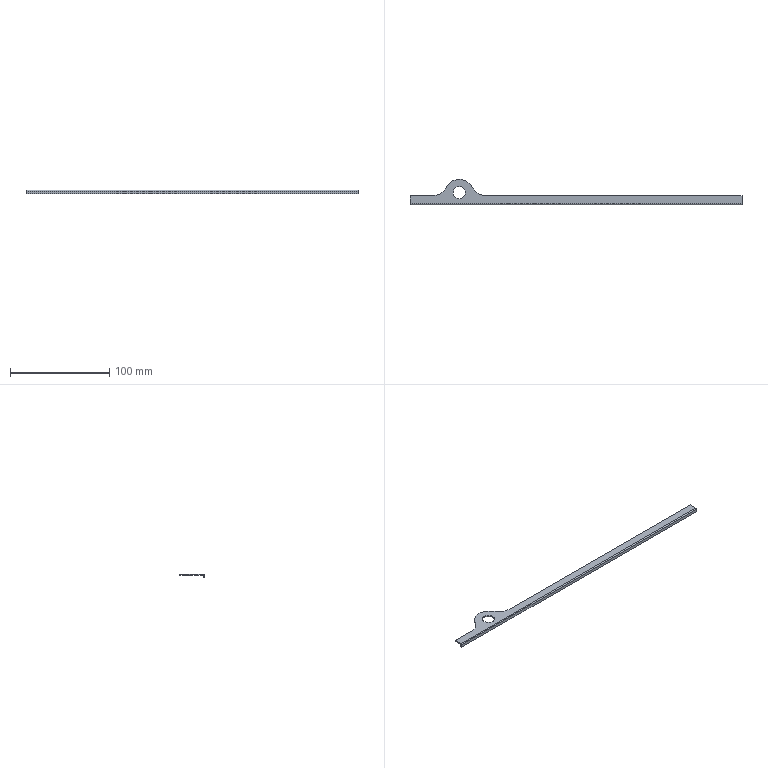Part | STEP file | gslz 2016.10.28-13_id1214_x_t | 1 solid | 14 faces | box 335 x 25.5 x 4 mm | volume 5252 mm3 | plane 9 | cylinder 5 | commonest cylinder face diameters 30 x3 2 x1 12.3 x1
STEP:
#1=CARTESIAN_POINT('',(0.,0.,0.));
#2=DIRECTION('',(0.,0.,1.));
#3=DIRECTION('',(1.,0.,0.));
#4=AXIS2_PLACEMENT_3D('',#1,#2,#3);
#5=CARTESIAN_POINT('',(-300.763,-257.,1.25));
#6=VERTEX_POINT('',#5);
#7=CARTESIAN_POINT('',(-42.345,-257.,1.25));
#8=VERTEX_POINT('',#7);
#9=CARTESIAN_POINT('',(-2539.517,-257.,1.25));
#10=DIRECTION('',(1.,0.,0.));
#11=VECTOR('',#10,1.);
#12=LINE('',#9,#11);
#13=CARTESIAN_POINT('',(-299.269,-257.,2.5));
#14=DIRECTION('',(0.,1.,0.));
#15=DIRECTION('',(-1.,0.,0.));
#16=AXIS2_PLACEMENT_3D('',#13,#14,#15);
#17=PLANE('',#16);
#18=CARTESIAN_POINT('',(2240.248,-1.25));
#19=DIRECTION('',(-1.,0.));
#20=VECTOR('',#19,1.);
#21=LINE('',#18,#20);
#22=(GEOMETRIC_REPRESENTATION_CONTEXT(2)PARAMETRIC_REPRESENTATION_CONTEXT()REPRESENTATION_CONTEXT('',''));
#23=DEFINITIONAL_REPRESENTATION('',(#21),#22);
#24=PCURVE('',#17,#23);
#25=CARTESIAN_POINT('',(-2539.517,-331.067,1.25));
#26=DIRECTION('',(0.,0.,1.));
#27=DIRECTION('',(-1.,0.,0.));
#28=AXIS2_PLACEMENT_3D('',#25,#26,#27);
#29=PLANE('',#28);
#30=CARTESIAN_POINT('',(0.,-74.067));
#31=DIRECTION('',(-1.,0.));
#32=VECTOR('',#31,1.);
#33=LINE('',#30,#32);
#34=(GEOMETRIC_REPRESENTATION_CONTEXT(2)PARAMETRIC_REPRESENTATION_CONTEXT()REPRESENTATION_CONTEXT('',''));
#35=DEFINITIONAL_REPRESENTATION('',(#33),#34);
#36=PCURVE('',#29,#35);
#37=SURFACE_CURVE('',#12,(#24,#36),.PCURVE_S1.);
#38=EDGE_CURVE('',#6,#8,#37,.T.);
#39=ORIENTED_EDGE('',*,*,#38,.T.);
#40=CARTESIAN_POINT('',(-42.345,-257.,0.));
#41=VERTEX_POINT('',#40);
#42=CARTESIAN_POINT('',(-42.345,-257.,-0.75));
#43=DIRECTION('',(0.,0.,1.));
#44=VECTOR('',#43,1.);
#45=LINE('',#42,#44);
#46=CARTESIAN_POINT('',(-256.924,-3.25));
#47=DIRECTION('',(0.,1.));
#48=VECTOR('',#47,1.);
#49=LINE('',#46,#48);
#50=(GEOMETRIC_REPRESENTATION_CONTEXT(2)PARAMETRIC_REPRESENTATION_CONTEXT()REPRESENTATION_CONTEXT('',''));
#51=DEFINITIONAL_REPRESENTATION('',(#49),#50);
#52=PCURVE('',#17,#51);
#53=CARTESIAN_POINT('',(-42.345,-261.5,-0.75));
#54=DIRECTION('',(1.,0.,0.));
#55=DIRECTION('',(0.,1.,0.));
#56=AXIS2_PLACEMENT_3D('',#53,#54,#55);
#57=PLANE('',#56);
#58=CARTESIAN_POINT('',(4.5,0.));
#59=DIRECTION('',(0.,1.));
#60=VECTOR('',#59,1.);
#61=LINE('',#58,#60);
#62=(GEOMETRIC_REPRESENTATION_CONTEXT(2)PARAMETRIC_REPRESENTATION_CONTEXT()REPRESENTATION_CONTEXT('',''));
#63=DEFINITIONAL_REPRESENTATION('',(#61),#62);
#64=PCURVE('',#57,#63);
#65=SURFACE_CURVE('',#45,(#52,#64),.PCURVE_S1.);
#66=EDGE_CURVE('',#41,#8,#65,.T.);
#67=ORIENTED_EDGE('',*,*,#66,.F.);
#68=CARTESIAN_POINT('',(-300.763,-257.,0.));
#69=VERTEX_POINT('',#68);
#70=CARTESIAN_POINT('',(-299.269,-257.,0.));
#71=DIRECTION('',(-1.,0.,0.));
#72=VECTOR('',#71,1.);
#73=LINE('',#70,#72);
#74=CARTESIAN_POINT('',(0.,-2.5));
#75=DIRECTION('',(1.,0.));
#76=VECTOR('',#75,1.);
#77=LINE('',#74,#76);
#78=(GEOMETRIC_REPRESENTATION_CONTEXT(2)PARAMETRIC_REPRESENTATION_CONTEXT()REPRESENTATION_CONTEXT('',''));
#79=DEFINITIONAL_REPRESENTATION('',(#77),#78);
#80=PCURVE('',#17,#79);
#81=CARTESIAN_POINT('',(-2539.517,-331.067,0.));
#82=DIRECTION('',(0.,0.,1.));
#83=DIRECTION('',(-1.,0.,0.));
#84=AXIS2_PLACEMENT_3D('',#81,#82,#83);
#85=PLANE('',#84);
#86=CARTESIAN_POINT('',(-2240.248,-74.067));
#87=DIRECTION('',(1.,0.));
#88=VECTOR('',#87,1.);
#89=LINE('',#86,#88);
#90=(GEOMETRIC_REPRESENTATION_CONTEXT(2)PARAMETRIC_REPRESENTATION_CONTEXT()REPRESENTATION_CONTEXT('',''));
#91=DEFINITIONAL_REPRESENTATION('',(#89),#90);
#92=PCURVE('',#85,#91);
#93=SURFACE_CURVE('',#73,(#80,#92),.PCURVE_S1.);
#94=EDGE_CURVE('',#41,#69,#93,.T.);
#95=ORIENTED_EDGE('',*,*,#94,.T.);
#96=CARTESIAN_POINT('',(-300.763,-257.,2.5));
#97=DIRECTION('',(0.,0.,1.));
#98=VECTOR('',#97,1.);
#99=LINE('',#96,#98);
#100=CARTESIAN_POINT('',(1.493,0.));
#101=DIRECTION('',(0.,1.));
#102=VECTOR('',#101,1.);
#103=LINE('',#100,#102);
#104=(GEOMETRIC_REPRESENTATION_CONTEXT(2)PARAMETRIC_REPRESENTATION_CONTEXT()REPRESENTATION_CONTEXT('',''));
#105=DEFINITIONAL_REPRESENTATION('',(#103),#104);
#106=PCURVE('',#17,#105);
#107=CARTESIAN_POINT('',(-300.763,-242.,2.5));
#108=DIRECTION('',(0.,0.,-1.));
#109=DIRECTION('',(1.,0.,0.));
#110=AXIS2_PLACEMENT_3D('',#107,#108,#109);
#111=CYLINDRICAL_SURFACE('',#110,15.);
#112=CARTESIAN_POINT('',(1.571,0.));
#113=DIRECTION('',(0.,-1.));
#114=VECTOR('',#113,1.);
#115=LINE('',#112,#114);
#116=(GEOMETRIC_REPRESENTATION_CONTEXT(2)PARAMETRIC_REPRESENTATION_CONTEXT()REPRESENTATION_CONTEXT('',''));
#117=DEFINITIONAL_REPRESENTATION('',(#115),#116);
#118=PCURVE('',#111,#117);
#119=SURFACE_CURVE('',#99,(#106,#118),.PCURVE_S1.);
#120=EDGE_CURVE('',#69,#6,#119,.T.);
#121=ORIENTED_EDGE('',*,*,#120,.T.);
#122=EDGE_LOOP('',(#39,#67,#95,#121));
#123=FACE_BOUND('',#122,.T.);
#124=ADVANCED_FACE('',(#123),#17,.T.);
#125=CARTESIAN_POINT('',(-333.704,-254.,1.25));
#126=VERTEX_POINT('',#125);
#127=CARTESIAN_POINT('',(-327.554,-254.,1.25));
#128=DIRECTION('',(0.,0.,1.));
#129=DIRECTION('',(-1.,0.,0.));
#130=AXIS2_PLACEMENT_3D('',#127,#128,#129);
#131=CIRCLE('',#130,6.15);
#132=CARTESIAN_POINT('',(-2211.964,-77.067));
#133=DIRECTION('',(1.,0.));
#134=AXIS2_PLACEMENT_2D('',#132,#133);
#135=CIRCLE('',#134,6.15);
#136=(GEOMETRIC_REPRESENTATION_CONTEXT(2)PARAMETRIC_REPRESENTATION_CONTEXT()REPRESENTATION_CONTEXT('',''));
#137=DEFINITIONAL_REPRESENTATION('',(#135),#136);
#138=PCURVE('',#29,#137);
#139=CARTESIAN_POINT('',(-327.554,-254.,2.5));
#140=DIRECTION('',(0.,0.,-1.));
#141=DIRECTION('',(1.,0.,0.));
#142=AXIS2_PLACEMENT_3D('',#139,#140,#141);
#143=CYLINDRICAL_SURFACE('',#142,6.15);
#144=CARTESIAN_POINT('',(9.425,1.25));
#145=DIRECTION('',(-1.,0.));
#146=VECTOR('',#145,1.);
#147=LINE('',#144,#146);
#148=(GEOMETRIC_REPRESENTATION_CONTEXT(2)PARAMETRIC_REPRESENTATION_CONTEXT()REPRESENTATION_CONTEXT('',''));
#149=DEFINITIONAL_REPRESENTATION('',(#147),#148);
#150=PCURVE('',#143,#149);
#151=SURFACE_CURVE('',#131,(#138,#150),.PCURVE_S1.);
#152=EDGE_CURVE('',#126,#126,#151,.T.);
#153=ORIENTED_EDGE('',*,*,#152,.F.);
#154=EDGE_LOOP('',(#153));
#155=FACE_BOUND('',#154,.T.);
#156=CARTESIAN_POINT('',(-377.345,-265.,1.25));
#157=VERTEX_POINT('',#156);
#158=CARTESIAN_POINT('',(-42.345,-265.,1.25));
#159=VERTEX_POINT('',#158);
#160=CARTESIAN_POINT('',(-119.75,-265.,1.25));
#161=DIRECTION('',(1.,0.,0.));
#162=VECTOR('',#161,1.);
#163=LINE('',#160,#162);
#164=CARTESIAN_POINT('',(-2419.767,-66.067));
#165=DIRECTION('',(-1.,0.));
#166=VECTOR('',#165,1.);
#167=LINE('',#164,#166);
#168=(GEOMETRIC_REPRESENTATION_CONTEXT(2)PARAMETRIC_REPRESENTATION_CONTEXT()REPRESENTATION_CONTEXT('',''));
#169=DEFINITIONAL_REPRESENTATION('',(#167),#168);
#170=PCURVE('',#29,#169);
#171=CARTESIAN_POINT('',(-2539.517,-265.,0.25));
#172=DIRECTION('',(1.,0.,0.));
#173=DIRECTION('',(0.,1.,0.));
#174=AXIS2_PLACEMENT_3D('',#171,#172,#173);
#175=CYLINDRICAL_SURFACE('',#174,1.);
#176=CARTESIAN_POINT('',(1.571,2419.767));
#177=DIRECTION('',(0.,1.));
#178=VECTOR('',#177,1.);
#179=LINE('',#176,#178);
#180=(GEOMETRIC_REPRESENTATION_CONTEXT(2)PARAMETRIC_REPRESENTATION_CONTEXT()REPRESENTATION_CONTEXT('',''));
#181=DEFINITIONAL_REPRESENTATION('',(#179),#180);
#182=PCURVE('',#175,#181);
#183=SURFACE_CURVE('',#163,(#170,#182),.PCURVE_S1.);
#184=EDGE_CURVE('',#157,#159,#183,.T.);
#185=ORIENTED_EDGE('',*,*,#184,.T.);
#186=CARTESIAN_POINT('',(-42.345,-331.067,1.25));
#187=DIRECTION('',(0.,1.,0.));
#188=VECTOR('',#187,1.);
#189=LINE('',#186,#188);
#190=CARTESIAN_POINT('',(-2497.172,0.));
#191=DIRECTION('',(0.,-1.));
#192=VECTOR('',#191,1.);
#193=LINE('',#190,#192);
#194=(GEOMETRIC_REPRESENTATION_CONTEXT(2)PARAMETRIC_REPRESENTATION_CONTEXT()REPRESENTATION_CONTEXT('',''));
#195=DEFINITIONAL_REPRESENTATION('',(#193),#194);
#196=PCURVE('',#29,#195);
#197=CARTESIAN_POINT('',(-69.567,2.));
#198=DIRECTION('',(1.,0.));
#199=VECTOR('',#198,1.);
#200=LINE('',#197,#199);
#201=(GEOMETRIC_REPRESENTATION_CONTEXT(2)PARAMETRIC_REPRESENTATION_CONTEXT()REPRESENTATION_CONTEXT('',''));
#202=DEFINITIONAL_REPRESENTATION('',(#200),#201);
#203=PCURVE('',#57,#202);
#204=SURFACE_CURVE('',#189,(#196,#203),.PCURVE_S1.);
#205=EDGE_CURVE('',#159,#8,#204,.T.);
#206=ORIENTED_EDGE('',*,*,#205,.T.);
#207=ORIENTED_EDGE('',*,*,#38,.F.);
#208=CARTESIAN_POINT('',(-314.158,-248.75,1.25));
#209=VERTEX_POINT('',#208);
#210=CARTESIAN_POINT('',(-300.763,-242.,1.25));
#211=DIRECTION('',(0.,0.,-1.));
#212=DIRECTION('',(-1.,0.,0.));
#213=AXIS2_PLACEMENT_3D('',#210,#211,#212);
#214=CIRCLE('',#213,15.);
#215=CARTESIAN_POINT('',(-2223.754,-89.067));
#216=CARTESIAN_POINT('',(-2223.754,-115.047));
#217=CARTESIAN_POINT('',(-2246.254,-102.057));
#218=CARTESIAN_POINT('',(-2268.754,-89.067));
#219=CARTESIAN_POINT('',(-2246.254,-76.076));
#220=CARTESIAN_POINT('',(-2223.754,-63.086));
#221=CARTESIAN_POINT('',(-2223.754,-89.067));
#222=(BOUNDED_CURVE()B_SPLINE_CURVE(2,(#215,#216,#217,#218,#219,#220,#221),.UNSPECIFIED.,.T.,.F.)B_SPLINE_CURVE_WITH_KNOTS((1,2,2,2,2,1),(-2.094,0.,2.094,4.189,6.283,8.378),.UNSPECIFIED.)CURVE()GEOMETRIC_REPRESENTATION_ITEM()RATIONAL_B_SPLINE_CURVE((1.,0.5,1.,0.5,1.,0.5,1.))REPRESENTATION_ITEM(''));
#223=(GEOMETRIC_REPRESENTATION_CONTEXT(2)PARAMETRIC_REPRESENTATION_CONTEXT()REPRESENTATION_CONTEXT('',''));
#224=DEFINITIONAL_REPRESENTATION('',(#222),#223);
#225=PCURVE('',#29,#224);
#226=CARTESIAN_POINT('',(-3.142,1.25));
#227=DIRECTION('',(1.,0.));
#228=VECTOR('',#227,1.);
#229=LINE('',#226,#228);
#230=(GEOMETRIC_REPRESENTATION_CONTEXT(2)PARAMETRIC_REPRESENTATION_CONTEXT()REPRESENTATION_CONTEXT('',''));
#231=DEFINITIONAL_REPRESENTATION('',(#229),#230);
#232=PCURVE('',#111,#231);
#233=SURFACE_CURVE('',#214,(#225,#232),.PCURVE_S1.);
#234=EDGE_CURVE('',#6,#209,#233,.T.);
#235=ORIENTED_EDGE('',*,*,#234,.T.);
#236=CARTESIAN_POINT('',(-340.949,-248.75,1.25));
#237=VERTEX_POINT('',#236);
#238=CARTESIAN_POINT('',(-327.554,-255.5,1.25));
#239=DIRECTION('',(0.,0.,1.));
#240=DIRECTION('',(-1.,0.,0.));
#241=AXIS2_PLACEMENT_3D('',#238,#239,#240);
#242=CIRCLE('',#241,15.);
#243=CARTESIAN_POINT('',(-2211.964,-75.567));
#244=DIRECTION('',(1.,0.));
#245=AXIS2_PLACEMENT_2D('',#243,#244);
#246=CIRCLE('',#245,15.);
#247=(GEOMETRIC_REPRESENTATION_CONTEXT(2)PARAMETRIC_REPRESENTATION_CONTEXT()REPRESENTATION_CONTEXT('',''));
#248=DEFINITIONAL_REPRESENTATION('',(#246),#247);
#249=PCURVE('',#29,#248);
#250=CARTESIAN_POINT('',(-327.554,-255.5,2.5));
#251=DIRECTION('',(0.,0.,-1.));
#252=DIRECTION('',(1.,0.,0.));
#253=AXIS2_PLACEMENT_3D('',#250,#251,#252);
#254=CYLINDRICAL_SURFACE('',#253,15.);
#255=CARTESIAN_POINT('',(9.425,1.25));
#256=DIRECTION('',(-1.,0.));
#257=VECTOR('',#256,1.);
#258=LINE('',#255,#257);
#259=(GEOMETRIC_REPRESENTATION_CONTEXT(2)PARAMETRIC_REPRESENTATION_CONTEXT()REPRESENTATION_CONTEXT('',''));
#260=DEFINITIONAL_REPRESENTATION('',(#258),#259);
#261=PCURVE('',#254,#260);
#262=SURFACE_CURVE('',#242,(#249,#261),.PCURVE_S1.);
#263=EDGE_CURVE('',#209,#237,#262,.T.);
#264=ORIENTED_EDGE('',*,*,#263,.T.);
#265=CARTESIAN_POINT('',(-354.345,-257.,1.25));
#266=VERTEX_POINT('',#265);
#267=CARTESIAN_POINT('',(-354.345,-242.,1.25));
#268=DIRECTION('',(0.,0.,-1.));
#269=DIRECTION('',(-1.,0.,0.));
#270=AXIS2_PLACEMENT_3D('',#267,#268,#269);
#271=CIRCLE('',#270,15.);
#272=CARTESIAN_POINT('',(-2170.173,-89.067));
#273=CARTESIAN_POINT('',(-2170.173,-115.047));
#274=CARTESIAN_POINT('',(-2192.673,-102.057));
#275=CARTESIAN_POINT('',(-2215.173,-89.067));
#276=CARTESIAN_POINT('',(-2192.673,-76.076));
#277=CARTESIAN_POINT('',(-2170.173,-63.086));
#278=CARTESIAN_POINT('',(-2170.173,-89.067));
#279=(BOUNDED_CURVE()B_SPLINE_CURVE(2,(#272,#273,#274,#275,#276,#277,#278),.UNSPECIFIED.,.T.,.F.)B_SPLINE_CURVE_WITH_KNOTS((1,2,2,2,2,1),(-2.094,0.,2.094,4.189,6.283,8.378),.UNSPECIFIED.)CURVE()GEOMETRIC_REPRESENTATION_ITEM()RATIONAL_B_SPLINE_CURVE((1.,0.5,1.,0.5,1.,0.5,1.))REPRESENTATION_ITEM(''));
#280=(GEOMETRIC_REPRESENTATION_CONTEXT(2)PARAMETRIC_REPRESENTATION_CONTEXT()REPRESENTATION_CONTEXT('',''));
#281=DEFINITIONAL_REPRESENTATION('',(#279),#280);
#282=PCURVE('',#29,#281);
#283=CARTESIAN_POINT('',(-354.345,-242.,2.5));
#284=DIRECTION('',(0.,0.,-1.));
#285=DIRECTION('',(1.,0.,0.));
#286=AXIS2_PLACEMENT_3D('',#283,#284,#285);
#287=CYLINDRICAL_SURFACE('',#286,15.);
#288=CARTESIAN_POINT('',(-3.142,1.25));
#289=DIRECTION('',(1.,0.));
#290=VECTOR('',#289,1.);
#291=LINE('',#288,#290);
#292=(GEOMETRIC_REPRESENTATION_CONTEXT(2)PARAMETRIC_REPRESENTATION_CONTEXT()REPRESENTATION_CONTEXT('',''));
#293=DEFINITIONAL_REPRESENTATION('',(#291),#292);
#294=PCURVE('',#287,#293);
#295=SURFACE_CURVE('',#271,(#282,#294),.PCURVE_S1.);
#296=EDGE_CURVE('',#237,#266,#295,.T.);
#297=ORIENTED_EDGE('',*,*,#296,.T.);
#298=CARTESIAN_POINT('',(-377.345,-257.,1.25));
#299=VERTEX_POINT('',#298);
#300=CARTESIAN_POINT('',(-2539.517,-257.,1.25));
#301=DIRECTION('',(1.,0.,0.));
#302=VECTOR('',#301,1.);
#303=LINE('',#300,#302);
#304=CARTESIAN_POINT('',(0.,-74.067));
#305=DIRECTION('',(-1.,0.));
#306=VECTOR('',#305,1.);
#307=LINE('',#304,#306);
#308=(GEOMETRIC_REPRESENTATION_CONTEXT(2)PARAMETRIC_REPRESENTATION_CONTEXT()REPRESENTATION_CONTEXT('',''));
#309=DEFINITIONAL_REPRESENTATION('',(#307),#308);
#310=PCURVE('',#29,#309);
#311=CARTESIAN_POINT('',(-334.709,-257.,0.));
#312=DIRECTION('',(0.,1.,0.));
#313=DIRECTION('',(0.,0.,-1.));
#314=AXIS2_PLACEMENT_3D('',#311,#312,#313);
#315=PLANE('',#314);
#316=CARTESIAN_POINT('',(-1.25,2204.808));
#317=DIRECTION('',(0.,-1.));
#318=VECTOR('',#317,1.);
#319=LINE('',#316,#318);
#320=(GEOMETRIC_REPRESENTATION_CONTEXT(2)PARAMETRIC_REPRESENTATION_CONTEXT()REPRESENTATION_CONTEXT('',''));
#321=DEFINITIONAL_REPRESENTATION('',(#319),#320);
#322=PCURVE('',#315,#321);
#323=SURFACE_CURVE('',#303,(#310,#322),.PCURVE_S1.);
#324=EDGE_CURVE('',#299,#266,#323,.T.);
#325=ORIENTED_EDGE('',*,*,#324,.F.);
#326=CARTESIAN_POINT('',(-377.345,319.067,1.25));
#327=DIRECTION('',(0.,1.,0.));
#328=VECTOR('',#327,1.);
#329=LINE('',#326,#328);
#330=CARTESIAN_POINT('',(-2162.172,-650.133));
#331=DIRECTION('',(0.,-1.));
#332=VECTOR('',#331,1.);
#333=LINE('',#330,#332);
#334=(GEOMETRIC_REPRESENTATION_CONTEXT(2)PARAMETRIC_REPRESENTATION_CONTEXT()REPRESENTATION_CONTEXT('',''));
#335=DEFINITIONAL_REPRESENTATION('',(#333),#334);
#336=PCURVE('',#29,#335);
#337=CARTESIAN_POINT('',(-377.345,-261.5,-0.75));
#338=DIRECTION('',(1.,0.,0.));
#339=DIRECTION('',(0.,1.,0.));
#340=AXIS2_PLACEMENT_3D('',#337,#338,#339);
#341=PLANE('',#340);
#342=CARTESIAN_POINT('',(580.567,2.));
#343=DIRECTION('',(1.,0.));
#344=VECTOR('',#343,1.);
#345=LINE('',#342,#344);
#346=(GEOMETRIC_REPRESENTATION_CONTEXT(2)PARAMETRIC_REPRESENTATION_CONTEXT()REPRESENTATION_CONTEXT('',''));
#347=DEFINITIONAL_REPRESENTATION('',(#345),#346);
#348=PCURVE('',#341,#347);
#349=SURFACE_CURVE('',#329,(#336,#348),.PCURVE_S1.);
#350=EDGE_CURVE('',#157,#299,#349,.T.);
#351=ORIENTED_EDGE('',*,*,#350,.F.);
#352=EDGE_LOOP('',(#185,#206,#207,#235,#264,#297,#325,#351));
#353=FACE_BOUND('',#352,.T.);
#354=ADVANCED_FACE('',(#155,#353),#29,.T.);
#355=CARTESIAN_POINT('',(-333.704,-254.,0.));
#356=VERTEX_POINT('',#355);
#357=CARTESIAN_POINT('',(-327.554,-254.,0.));
#358=DIRECTION('',(0.,0.,-1.));
#359=DIRECTION('',(-1.,0.,0.));
#360=AXIS2_PLACEMENT_3D('',#357,#358,#359);
#361=CIRCLE('',#360,6.15);
#362=CARTESIAN_POINT('',(-2205.814,-77.067));
#363=CARTESIAN_POINT('',(-2205.814,-87.719));
#364=CARTESIAN_POINT('',(-2215.039,-82.393));
#365=CARTESIAN_POINT('',(-2224.264,-77.067));
#366=CARTESIAN_POINT('',(-2215.039,-71.741));
#367=CARTESIAN_POINT('',(-2205.814,-66.415));
#368=CARTESIAN_POINT('',(-2205.814,-77.067));
#369=(BOUNDED_CURVE()B_SPLINE_CURVE(2,(#362,#363,#364,#365,#366,#367,#368),.UNSPECIFIED.,.T.,.F.)B_SPLINE_CURVE_WITH_KNOTS((1,2,2,2,2,1),(-2.094,0.,2.094,4.189,6.283,8.378),.UNSPECIFIED.)CURVE()GEOMETRIC_REPRESENTATION_ITEM()RATIONAL_B_SPLINE_CURVE((1.,0.5,1.,0.5,1.,0.5,1.))REPRESENTATION_ITEM(''));
#370=(GEOMETRIC_REPRESENTATION_CONTEXT(2)PARAMETRIC_REPRESENTATION_CONTEXT()REPRESENTATION_CONTEXT('',''));
#371=DEFINITIONAL_REPRESENTATION('',(#369),#370);
#372=PCURVE('',#85,#371);
#373=CARTESIAN_POINT('',(3.142,2.5));
#374=DIRECTION('',(1.,0.));
#375=VECTOR('',#374,1.);
#376=LINE('',#373,#375);
#377=(GEOMETRIC_REPRESENTATION_CONTEXT(2)PARAMETRIC_REPRESENTATION_CONTEXT()REPRESENTATION_CONTEXT('',''));
#378=DEFINITIONAL_REPRESENTATION('',(#376),#377);
#379=PCURVE('',#143,#378);
#380=SURFACE_CURVE('',#361,(#372,#379),.PCURVE_S1.);
#381=EDGE_CURVE('',#356,#356,#380,.T.);
#382=ORIENTED_EDGE('',*,*,#381,.F.);
#383=EDGE_LOOP('',(#382));
#384=FACE_BOUND('',#383,.T.);
#385=ORIENTED_EDGE('',*,*,#94,.F.);
#386=CARTESIAN_POINT('',(-42.345,-264.75,0.));
#387=VERTEX_POINT('',#386);
#388=CARTESIAN_POINT('',(-42.345,-261.5,0.));
#389=DIRECTION('',(0.,-1.,0.));
#390=VECTOR('',#389,1.);
#391=LINE('',#388,#390);
#392=CARTESIAN_POINT('',(-2497.172,-69.567));
#393=DIRECTION('',(0.,1.));
#394=VECTOR('',#393,1.);
#395=LINE('',#392,#394);
#396=(GEOMETRIC_REPRESENTATION_CONTEXT(2)PARAMETRIC_REPRESENTATION_CONTEXT()REPRESENTATION_CONTEXT('',''));
#397=DEFINITIONAL_REPRESENTATION('',(#395),#396);
#398=PCURVE('',#85,#397);
#399=CARTESIAN_POINT('',(0.,0.75));
#400=DIRECTION('',(-1.,0.));
#401=VECTOR('',#400,1.);
#402=LINE('',#399,#401);
#403=(GEOMETRIC_REPRESENTATION_CONTEXT(2)PARAMETRIC_REPRESENTATION_CONTEXT()REPRESENTATION_CONTEXT('',''));
#404=DEFINITIONAL_REPRESENTATION('',(#402),#403);
#405=PCURVE('',#57,#404);
#406=SURFACE_CURVE('',#391,(#398,#405),.PCURVE_S1.);
#407=EDGE_CURVE('',#41,#387,#406,.T.);
#408=ORIENTED_EDGE('',*,*,#407,.T.);
#409=CARTESIAN_POINT('',(-377.345,-264.75,0.));
#410=VERTEX_POINT('',#409);
#411=CARTESIAN_POINT('',(-2299.851,-264.75,0.));
#412=DIRECTION('',(1.,0.,0.));
#413=VECTOR('',#412,1.);
#414=LINE('',#411,#413);
#415=CARTESIAN_POINT('',(-239.666,-66.317));
#416=DIRECTION('',(-1.,0.));
#417=VECTOR('',#416,1.);
#418=LINE('',#415,#417);
#419=(GEOMETRIC_REPRESENTATION_CONTEXT(2)PARAMETRIC_REPRESENTATION_CONTEXT()REPRESENTATION_CONTEXT('',''));
#420=DEFINITIONAL_REPRESENTATION('',(#418),#419);
#421=PCURVE('',#85,#420);
#422=CARTESIAN_POINT('',(-2299.851,-264.75,-135.834));
#423=DIRECTION('',(0.,-1.,0.));
#424=DIRECTION('',(-1.,0.,0.));
#425=AXIS2_PLACEMENT_3D('',#422,#423,#424);
#426=PLANE('',#425);
#427=CARTESIAN_POINT('',(0.,-135.834));
#428=DIRECTION('',(-1.,0.));
#429=VECTOR('',#428,1.);
#430=LINE('',#427,#429);
#431=(GEOMETRIC_REPRESENTATION_CONTEXT(2)PARAMETRIC_REPRESENTATION_CONTEXT()REPRESENTATION_CONTEXT('',''));
#432=DEFINITIONAL_REPRESENTATION('',(#430),#431);
#433=PCURVE('',#426,#432);
#434=SURFACE_CURVE('',#414,(#421,#433),.PCURVE_S1.);
#435=EDGE_CURVE('',#410,#387,#434,.T.);
#436=ORIENTED_EDGE('',*,*,#435,.F.);
#437=CARTESIAN_POINT('',(-377.345,-257.,0.));
#438=VERTEX_POINT('',#437);
#439=CARTESIAN_POINT('',(-377.345,319.067,0.));
#440=DIRECTION('',(0.,-1.,0.));
#441=VECTOR('',#440,1.);
#442=LINE('',#439,#441);
#443=CARTESIAN_POINT('',(-2162.172,-650.133));
#444=DIRECTION('',(0.,1.));
#445=VECTOR('',#444,1.);
#446=LINE('',#443,#445);
#447=(GEOMETRIC_REPRESENTATION_CONTEXT(2)PARAMETRIC_REPRESENTATION_CONTEXT()REPRESENTATION_CONTEXT('',''));
#448=DEFINITIONAL_REPRESENTATION('',(#446),#447);
#449=PCURVE('',#85,#448);
#450=CARTESIAN_POINT('',(580.567,0.75));
#451=DIRECTION('',(-1.,0.));
#452=VECTOR('',#451,1.);
#453=LINE('',#450,#452);
#454=(GEOMETRIC_REPRESENTATION_CONTEXT(2)PARAMETRIC_REPRESENTATION_CONTEXT()REPRESENTATION_CONTEXT('',''));
#455=DEFINITIONAL_REPRESENTATION('',(#453),#454);
#456=PCURVE('',#341,#455);
#457=SURFACE_CURVE('',#442,(#449,#456),.PCURVE_S1.);
#458=EDGE_CURVE('',#438,#410,#457,.T.);
#459=ORIENTED_EDGE('',*,*,#458,.F.);
#460=CARTESIAN_POINT('',(-354.345,-257.,0.));
#461=VERTEX_POINT('',#460);
#462=CARTESIAN_POINT('',(-334.709,-257.,0.));
#463=DIRECTION('',(-1.,0.,0.));
#464=VECTOR('',#463,1.);
#465=LINE('',#462,#464);
#466=CARTESIAN_POINT('',(-2204.808,-74.067));
#467=DIRECTION('',(1.,0.));
#468=VECTOR('',#467,1.);
#469=LINE('',#466,#468);
#470=(GEOMETRIC_REPRESENTATION_CONTEXT(2)PARAMETRIC_REPRESENTATION_CONTEXT()REPRESENTATION_CONTEXT('',''));
#471=DEFINITIONAL_REPRESENTATION('',(#469),#470);
#472=PCURVE('',#85,#471);
#473=CARTESIAN_POINT('',(0.,0.));
#474=DIRECTION('',(0.,1.));
#475=VECTOR('',#474,1.);
#476=LINE('',#473,#475);
#477=(GEOMETRIC_REPRESENTATION_CONTEXT(2)PARAMETRIC_REPRESENTATION_CONTEXT()REPRESENTATION_CONTEXT('',''));
#478=DEFINITIONAL_REPRESENTATION('',(#476),#477);
#479=PCURVE('',#315,#478);
#480=SURFACE_CURVE('',#465,(#472,#479),.PCURVE_S1.);
#481=EDGE_CURVE('',#461,#438,#480,.T.);
#482=ORIENTED_EDGE('',*,*,#481,.F.);
#483=CARTESIAN_POINT('',(-340.949,-248.75,0.));
#484=VERTEX_POINT('',#483);
#485=CARTESIAN_POINT('',(-354.345,-242.,0.));
#486=DIRECTION('',(0.,0.,1.));
#487=DIRECTION('',(-1.,0.,0.));
#488=AXIS2_PLACEMENT_3D('',#485,#486,#487);
#489=CIRCLE('',#488,15.);
#490=CARTESIAN_POINT('',(-2185.173,-89.067));
#491=DIRECTION('',(1.,0.));
#492=AXIS2_PLACEMENT_2D('',#490,#491);
#493=CIRCLE('',#492,15.);
#494=(GEOMETRIC_REPRESENTATION_CONTEXT(2)PARAMETRIC_REPRESENTATION_CONTEXT()REPRESENTATION_CONTEXT('',''));
#495=DEFINITIONAL_REPRESENTATION('',(#493),#494);
#496=PCURVE('',#85,#495);
#497=CARTESIAN_POINT('',(3.142,2.5));
#498=DIRECTION('',(-1.,0.));
#499=VECTOR('',#498,1.);
#500=LINE('',#497,#499);
#501=(GEOMETRIC_REPRESENTATION_CONTEXT(2)PARAMETRIC_REPRESENTATION_CONTEXT()REPRESENTATION_CONTEXT('',''));
#502=DEFINITIONAL_REPRESENTATION('',(#500),#501);
#503=PCURVE('',#287,#502);
#504=SURFACE_CURVE('',#489,(#496,#503),.PCURVE_S1.);
#505=EDGE_CURVE('',#461,#484,#504,.T.);
#506=ORIENTED_EDGE('',*,*,#505,.T.);
#507=CARTESIAN_POINT('',(-314.158,-248.75,0.));
#508=VERTEX_POINT('',#507);
#509=CARTESIAN_POINT('',(-327.554,-255.5,0.));
#510=DIRECTION('',(0.,0.,-1.));
#511=DIRECTION('',(-1.,0.,0.));
#512=AXIS2_PLACEMENT_3D('',#509,#510,#511);
#513=CIRCLE('',#512,15.);
#514=CARTESIAN_POINT('',(-2196.964,-75.567));
#515=CARTESIAN_POINT('',(-2196.964,-101.547));
#516=CARTESIAN_POINT('',(-2219.464,-88.557));
#517=CARTESIAN_POINT('',(-2241.964,-75.567));
#518=CARTESIAN_POINT('',(-2219.464,-62.576));
#519=CARTESIAN_POINT('',(-2196.964,-49.586));
#520=CARTESIAN_POINT('',(-2196.964,-75.567));
#521=(BOUNDED_CURVE()B_SPLINE_CURVE(2,(#514,#515,#516,#517,#518,#519,#520),.UNSPECIFIED.,.T.,.F.)B_SPLINE_CURVE_WITH_KNOTS((1,2,2,2,2,1),(-2.094,0.,2.094,4.189,6.283,8.378),.UNSPECIFIED.)CURVE()GEOMETRIC_REPRESENTATION_ITEM()RATIONAL_B_SPLINE_CURVE((1.,0.5,1.,0.5,1.,0.5,1.))REPRESENTATION_ITEM(''));
#522=(GEOMETRIC_REPRESENTATION_CONTEXT(2)PARAMETRIC_REPRESENTATION_CONTEXT()REPRESENTATION_CONTEXT('',''));
#523=DEFINITIONAL_REPRESENTATION('',(#521),#522);
#524=PCURVE('',#85,#523);
#525=CARTESIAN_POINT('',(3.142,2.5));
#526=DIRECTION('',(1.,0.));
#527=VECTOR('',#526,1.);
#528=LINE('',#525,#527);
#529=(GEOMETRIC_REPRESENTATION_CONTEXT(2)PARAMETRIC_REPRESENTATION_CONTEXT()REPRESENTATION_CONTEXT('',''));
#530=DEFINITIONAL_REPRESENTATION('',(#528),#529);
#531=PCURVE('',#254,#530);
#532=SURFACE_CURVE('',#513,(#524,#531),.PCURVE_S1.);
#533=EDGE_CURVE('',#484,#508,#532,.T.);
#534=ORIENTED_EDGE('',*,*,#533,.T.);
#535=CARTESIAN_POINT('',(-300.763,-242.,0.));
#536=DIRECTION('',(0.,0.,1.));
#537=DIRECTION('',(-1.,0.,0.));
#538=AXIS2_PLACEMENT_3D('',#535,#536,#537);
#539=CIRCLE('',#538,15.);
#540=CARTESIAN_POINT('',(-2238.754,-89.067));
#541=DIRECTION('',(1.,0.));
#542=AXIS2_PLACEMENT_2D('',#540,#541);
#543=CIRCLE('',#542,15.);
#544=(GEOMETRIC_REPRESENTATION_CONTEXT(2)PARAMETRIC_REPRESENTATION_CONTEXT()REPRESENTATION_CONTEXT('',''));
#545=DEFINITIONAL_REPRESENTATION('',(#543),#544);
#546=PCURVE('',#85,#545);
#547=CARTESIAN_POINT('',(3.142,2.5));
#548=DIRECTION('',(-1.,0.));
#549=VECTOR('',#548,1.);
#550=LINE('',#547,#549);
#551=(GEOMETRIC_REPRESENTATION_CONTEXT(2)PARAMETRIC_REPRESENTATION_CONTEXT()REPRESENTATION_CONTEXT('',''));
#552=DEFINITIONAL_REPRESENTATION('',(#550),#551);
#553=PCURVE('',#111,#552);
#554=SURFACE_CURVE('',#539,(#546,#553),.PCURVE_S1.);
#555=EDGE_CURVE('',#508,#69,#554,.T.);
#556=ORIENTED_EDGE('',*,*,#555,.T.);
#557=EDGE_LOOP('',(#385,#408,#436,#459,#482,#506,#534,#556));
#558=FACE_BOUND('',#557,.T.);
#559=ADVANCED_FACE('',(#384,#558),#85,.F.);
#560=CARTESIAN_POINT('',(-42.345,-264.75,-2.75));
#561=VERTEX_POINT('',#560);
#562=CARTESIAN_POINT('',(-377.345,-264.75,-2.75));
#563=VERTEX_POINT('',#562);
#564=CARTESIAN_POINT('',(974.074,-264.75,-2.75));
#565=DIRECTION('',(-1.,0.,0.));
#566=VECTOR('',#565,1.);
#567=LINE('',#564,#566);
#568=CARTESIAN_POINT('',(974.074,-266.,-2.75));
#569=DIRECTION('',(0.,0.,1.));
#570=DIRECTION('',(1.,0.,0.));
#571=AXIS2_PLACEMENT_3D('',#568,#569,#570);
#572=PLANE('',#571);
#573=CARTESIAN_POINT('',(0.,1.25));
#574=DIRECTION('',(-1.,0.));
#575=VECTOR('',#574,1.);
#576=LINE('',#573,#575);
#577=(GEOMETRIC_REPRESENTATION_CONTEXT(2)PARAMETRIC_REPRESENTATION_CONTEXT()REPRESENTATION_CONTEXT('',''));
#578=DEFINITIONAL_REPRESENTATION('',(#576),#577);
#579=PCURVE('',#572,#578);
#580=CARTESIAN_POINT('',(-3273.925,-133.084));
#581=DIRECTION('',(1.,0.));
#582=VECTOR('',#581,1.);
#583=LINE('',#580,#582);
#584=(GEOMETRIC_REPRESENTATION_CONTEXT(2)PARAMETRIC_REPRESENTATION_CONTEXT()REPRESENTATION_CONTEXT('',''));
#585=DEFINITIONAL_REPRESENTATION('',(#583),#584);
#586=PCURVE('',#426,#585);
#587=SURFACE_CURVE('',#567,(#579,#586),.PCURVE_S1.);
#588=EDGE_CURVE('',#561,#563,#587,.T.);
#589=ORIENTED_EDGE('',*,*,#588,.F.);
#590=CARTESIAN_POINT('',(-42.345,-266.,-2.75));
#591=VERTEX_POINT('',#590);
#592=CARTESIAN_POINT('',(-42.345,-266.,-2.75));
#593=DIRECTION('',(0.,1.,0.));
#594=VECTOR('',#593,1.);
#595=LINE('',#592,#594);
#596=CARTESIAN_POINT('',(-1016.419,0.));
#597=DIRECTION('',(0.,1.));
#598=VECTOR('',#597,1.);
#599=LINE('',#596,#598);
#600=(GEOMETRIC_REPRESENTATION_CONTEXT(2)PARAMETRIC_REPRESENTATION_CONTEXT()REPRESENTATION_CONTEXT('',''));
#601=DEFINITIONAL_REPRESENTATION('',(#599),#600);
#602=PCURVE('',#572,#601);
#603=CARTESIAN_POINT('',(-4.5,-2.));
#604=DIRECTION('',(1.,0.));
#605=VECTOR('',#604,1.);
#606=LINE('',#603,#605);
#607=(GEOMETRIC_REPRESENTATION_CONTEXT(2)PARAMETRIC_REPRESENTATION_CONTEXT()REPRESENTATION_CONTEXT('',''));
#608=DEFINITIONAL_REPRESENTATION('',(#606),#607);
#609=PCURVE('',#57,#608);
#610=SURFACE_CURVE('',#595,(#602,#609),.PCURVE_S1.);
#611=EDGE_CURVE('',#591,#561,#610,.T.);
#612=ORIENTED_EDGE('',*,*,#611,.F.);
#613=CARTESIAN_POINT('',(-377.345,-266.,-2.75));
#614=VERTEX_POINT('',#613);
#615=CARTESIAN_POINT('',(974.074,-266.,-2.75));
#616=DIRECTION('',(-1.,0.,0.));
#617=VECTOR('',#616,1.);
#618=LINE('',#615,#617);
#619=CARTESIAN_POINT('',(0.,0.));
#620=DIRECTION('',(-1.,0.));
#621=VECTOR('',#620,1.);
#622=LINE('',#619,#621);
#623=(GEOMETRIC_REPRESENTATION_CONTEXT(2)PARAMETRIC_REPRESENTATION_CONTEXT()REPRESENTATION_CONTEXT('',''));
#624=DEFINITIONAL_REPRESENTATION('',(#622),#623);
#625=PCURVE('',#572,#624);
#626=CARTESIAN_POINT('',(-287.351,-266.,0.625));
#627=DIRECTION('',(0.,-1.,0.));
#628=DIRECTION('',(-1.,0.,0.));
#629=AXIS2_PLACEMENT_3D('',#626,#627,#628);
#630=PLANE('',#629);
#631=CARTESIAN_POINT('',(-1261.425,3.375));
#632=DIRECTION('',(1.,0.));
#633=VECTOR('',#632,1.);
#634=LINE('',#631,#633);
#635=(GEOMETRIC_REPRESENTATION_CONTEXT(2)PARAMETRIC_REPRESENTATION_CONTEXT()REPRESENTATION_CONTEXT('',''));
#636=DEFINITIONAL_REPRESENTATION('',(#634),#635);
#637=PCURVE('',#630,#636);
#638=SURFACE_CURVE('',#618,(#625,#637),.PCURVE_S1.);
#639=EDGE_CURVE('',#591,#614,#638,.T.);
#640=ORIENTED_EDGE('',*,*,#639,.T.);
#641=CARTESIAN_POINT('',(-377.345,-266.,-2.75));
#642=DIRECTION('',(0.,-1.,0.));
#643=VECTOR('',#642,1.);
#644=LINE('',#641,#643);
#645=CARTESIAN_POINT('',(-1351.419,0.));
#646=DIRECTION('',(0.,-1.));
#647=VECTOR('',#646,1.);
#648=LINE('',#645,#647);
#649=(GEOMETRIC_REPRESENTATION_CONTEXT(2)PARAMETRIC_REPRESENTATION_CONTEXT()REPRESENTATION_CONTEXT('',''));
#650=DEFINITIONAL_REPRESENTATION('',(#648),#649);
#651=PCURVE('',#572,#650);
#652=CARTESIAN_POINT('',(-4.5,-2.));
#653=DIRECTION('',(-1.,0.));
#654=VECTOR('',#653,1.);
#655=LINE('',#652,#654);
#656=(GEOMETRIC_REPRESENTATION_CONTEXT(2)PARAMETRIC_REPRESENTATION_CONTEXT()REPRESENTATION_CONTEXT('',''));
#657=DEFINITIONAL_REPRESENTATION('',(#655),#656);
#658=PCURVE('',#341,#657);
#659=SURFACE_CURVE('',#644,(#651,#658),.PCURVE_S1.);
#660=EDGE_CURVE('',#563,#614,#659,.T.);
#661=ORIENTED_EDGE('',*,*,#660,.F.);
#662=EDGE_LOOP('',(#589,#612,#640,#661));
#663=FACE_BOUND('',#662,.T.);
#664=ADVANCED_FACE('',(#663),#572,.F.);
#665=ORIENTED_EDGE('',*,*,#639,.F.);
#666=CARTESIAN_POINT('',(-42.345,-266.,0.25));
#667=VERTEX_POINT('',#666);
#668=CARTESIAN_POINT('',(-42.345,-266.,-0.75));
#669=DIRECTION('',(0.,0.,-1.));
#670=VECTOR('',#669,1.);
#671=LINE('',#668,#670);
#672=CARTESIAN_POINT('',(-245.006,1.375));
#673=DIRECTION('',(0.,1.));
#674=VECTOR('',#673,1.);
#675=LINE('',#672,#674);
#676=(GEOMETRIC_REPRESENTATION_CONTEXT(2)PARAMETRIC_REPRESENTATION_CONTEXT()REPRESENTATION_CONTEXT('',''));
#677=DEFINITIONAL_REPRESENTATION('',(#675),#676);
#678=PCURVE('',#630,#677);
#679=CARTESIAN_POINT('',(-4.5,0.));
#680=DIRECTION('',(0.,-1.));
#681=VECTOR('',#680,1.);
#682=LINE('',#679,#681);
#683=(GEOMETRIC_REPRESENTATION_CONTEXT(2)PARAMETRIC_REPRESENTATION_CONTEXT()REPRESENTATION_CONTEXT('',''));
#684=DEFINITIONAL_REPRESENTATION('',(#682),#683);
#685=PCURVE('',#57,#684);
#686=SURFACE_CURVE('',#671,(#678,#685),.PCURVE_S1.);
#687=EDGE_CURVE('',#667,#591,#686,.T.);
#688=ORIENTED_EDGE('',*,*,#687,.F.);
#689=CARTESIAN_POINT('',(-377.345,-266.,0.25));
#690=VERTEX_POINT('',#689);
#691=CARTESIAN_POINT('',(-459.851,-266.,0.25));
#692=DIRECTION('',(-1.,0.,0.));
#693=VECTOR('',#692,1.);
#694=LINE('',#691,#693);
#695=CARTESIAN_POINT('',(172.5,0.375));
#696=DIRECTION('',(1.,0.));
#697=VECTOR('',#696,1.);
#698=LINE('',#695,#697);
#699=(GEOMETRIC_REPRESENTATION_CONTEXT(2)PARAMETRIC_REPRESENTATION_CONTEXT()REPRESENTATION_CONTEXT('',''));
#700=DEFINITIONAL_REPRESENTATION('',(#698),#699);
#701=PCURVE('',#630,#700);
#702=CARTESIAN_POINT('',(3.142,2079.666));
#703=DIRECTION('',(0.,-1.));
#704=VECTOR('',#703,1.);
#705=LINE('',#702,#704);
#706=(GEOMETRIC_REPRESENTATION_CONTEXT(2)PARAMETRIC_REPRESENTATION_CONTEXT()REPRESENTATION_CONTEXT('',''));
#707=DEFINITIONAL_REPRESENTATION('',(#705),#706);
#708=PCURVE('',#175,#707);
#709=SURFACE_CURVE('',#694,(#701,#708),.PCURVE_S1.);
#710=EDGE_CURVE('',#667,#690,#709,.T.);
#711=ORIENTED_EDGE('',*,*,#710,.T.);
#712=CARTESIAN_POINT('',(-377.345,-266.,0.625));
#713=DIRECTION('',(0.,0.,-1.));
#714=VECTOR('',#713,1.);
#715=LINE('',#712,#714);
#716=CARTESIAN_POINT('',(89.994,0.));
#717=DIRECTION('',(0.,1.));
#718=VECTOR('',#717,1.);
#719=LINE('',#716,#718);
#720=(GEOMETRIC_REPRESENTATION_CONTEXT(2)PARAMETRIC_REPRESENTATION_CONTEXT()REPRESENTATION_CONTEXT('',''));
#721=DEFINITIONAL_REPRESENTATION('',(#719),#720);
#722=PCURVE('',#630,#721);
#723=CARTESIAN_POINT('',(-4.5,1.375));
#724=DIRECTION('',(0.,-1.));
#725=VECTOR('',#724,1.);
#726=LINE('',#723,#725);
#727=(GEOMETRIC_REPRESENTATION_CONTEXT(2)PARAMETRIC_REPRESENTATION_CONTEXT()REPRESENTATION_CONTEXT('',''));
#728=DEFINITIONAL_REPRESENTATION('',(#726),#727);
#729=PCURVE('',#341,#728);
#730=SURFACE_CURVE('',#715,(#722,#729),.PCURVE_S1.);
#731=EDGE_CURVE('',#690,#614,#730,.T.);
#732=ORIENTED_EDGE('',*,*,#731,.T.);
#733=EDGE_LOOP('',(#665,#688,#711,#732));
#734=FACE_BOUND('',#733,.T.);
#735=ADVANCED_FACE('',(#734),#630,.T.);
#736=ORIENTED_EDGE('',*,*,#435,.T.);
#737=CARTESIAN_POINT('',(-42.345,-264.75,-0.75));
#738=DIRECTION('',(0.,0.,-1.));
#739=VECTOR('',#738,1.);
#740=LINE('',#737,#739);
#741=CARTESIAN_POINT('',(-2257.506,-135.084));
#742=DIRECTION('',(0.,1.));
#743=VECTOR('',#742,1.);
#744=LINE('',#741,#743);
#745=(GEOMETRIC_REPRESENTATION_CONTEXT(2)PARAMETRIC_REPRESENTATION_CONTEXT()REPRESENTATION_CONTEXT('',''));
#746=DEFINITIONAL_REPRESENTATION('',(#744),#745);
#747=PCURVE('',#426,#746);
#748=CARTESIAN_POINT('',(-3.25,0.));
#749=DIRECTION('',(0.,-1.));
#750=VECTOR('',#749,1.);
#751=LINE('',#748,#750);
#752=(GEOMETRIC_REPRESENTATION_CONTEXT(2)PARAMETRIC_REPRESENTATION_CONTEXT()REPRESENTATION_CONTEXT('',''));
#753=DEFINITIONAL_REPRESENTATION('',(#751),#752);
#754=PCURVE('',#57,#753);
#755=SURFACE_CURVE('',#740,(#747,#754),.PCURVE_S1.);
#756=EDGE_CURVE('',#387,#561,#755,.T.);
#757=ORIENTED_EDGE('',*,*,#756,.T.);
#758=ORIENTED_EDGE('',*,*,#588,.T.);
#759=CARTESIAN_POINT('',(-377.345,-264.75,-135.834));
#760=DIRECTION('',(0.,0.,-1.));
#761=VECTOR('',#760,1.);
#762=LINE('',#759,#761);
#763=CARTESIAN_POINT('',(-1922.506,0.));
#764=DIRECTION('',(0.,1.));
#765=VECTOR('',#764,1.);
#766=LINE('',#763,#765);
#767=(GEOMETRIC_REPRESENTATION_CONTEXT(2)PARAMETRIC_REPRESENTATION_CONTEXT()REPRESENTATION_CONTEXT('',''));
#768=DEFINITIONAL_REPRESENTATION('',(#766),#767);
#769=PCURVE('',#426,#768);
#770=CARTESIAN_POINT('',(-3.25,-135.084));
#771=DIRECTION('',(0.,-1.));
#772=VECTOR('',#771,1.);
#773=LINE('',#770,#772);
#774=(GEOMETRIC_REPRESENTATION_CONTEXT(2)PARAMETRIC_REPRESENTATION_CONTEXT()REPRESENTATION_CONTEXT('',''));
#775=DEFINITIONAL_REPRESENTATION('',(#773),#774);
#776=PCURVE('',#341,#775);
#777=SURFACE_CURVE('',#762,(#769,#776),.PCURVE_S1.);
#778=EDGE_CURVE('',#410,#563,#777,.T.);
#779=ORIENTED_EDGE('',*,*,#778,.F.);
#780=EDGE_LOOP('',(#736,#757,#758,#779));
#781=FACE_BOUND('',#780,.T.);
#782=ADVANCED_FACE('',(#781),#426,.F.);
#783=ORIENTED_EDGE('',*,*,#710,.F.);
#784=CARTESIAN_POINT('',(-42.345,-265.,0.25));
#785=DIRECTION('',(-1.,0.,0.));
#786=DIRECTION('',(0.,1.,0.));
#787=AXIS2_PLACEMENT_3D('',#784,#785,#786);
#788=CIRCLE('',#787,1.);
#789=CARTESIAN_POINT('',(6.283,2497.172));
#790=DIRECTION('',(-1.,0.));
#791=VECTOR('',#790,1.);
#792=LINE('',#789,#791);
#793=(GEOMETRIC_REPRESENTATION_CONTEXT(2)PARAMETRIC_REPRESENTATION_CONTEXT()REPRESENTATION_CONTEXT('',''));
#794=DEFINITIONAL_REPRESENTATION('',(#792),#793);
#795=PCURVE('',#175,#794);
#796=CARTESIAN_POINT('',(-2.5,1.));
#797=CARTESIAN_POINT('',(-2.5,-0.7321));
#798=CARTESIAN_POINT('',(-4.,0.134));
#799=CARTESIAN_POINT('',(-5.5,1.));
#800=CARTESIAN_POINT('',(-4.,1.866));
#801=CARTESIAN_POINT('',(-2.5,2.732));
#802=CARTESIAN_POINT('',(-2.5,1.));
#803=(BOUNDED_CURVE()B_SPLINE_CURVE(2,(#796,#797,#798,#799,#800,#801,#802),.UNSPECIFIED.,.T.,.F.)B_SPLINE_CURVE_WITH_KNOTS((1,2,2,2,2,1),(-2.094,0.,2.094,4.189,6.283,8.378),.UNSPECIFIED.)CURVE()GEOMETRIC_REPRESENTATION_ITEM()RATIONAL_B_SPLINE_CURVE((1.,0.5,1.,0.5,1.,0.5,1.))REPRESENTATION_ITEM(''));
#804=(GEOMETRIC_REPRESENTATION_CONTEXT(2)PARAMETRIC_REPRESENTATION_CONTEXT()REPRESENTATION_CONTEXT('',''));
#805=DEFINITIONAL_REPRESENTATION('',(#803),#804);
#806=PCURVE('',#57,#805);
#807=SURFACE_CURVE('',#788,(#795,#806),.PCURVE_S1.);
#808=EDGE_CURVE('',#667,#159,#807,.T.);
#809=ORIENTED_EDGE('',*,*,#808,.T.);
#810=ORIENTED_EDGE('',*,*,#184,.F.);
#811=CARTESIAN_POINT('',(-377.345,-265.,0.25));
#812=DIRECTION('',(-1.,0.,0.));
#813=DIRECTION('',(0.,1.,0.));
#814=AXIS2_PLACEMENT_3D('',#811,#812,#813);
#815=CIRCLE('',#814,1.);
#816=CARTESIAN_POINT('',(6.283,2162.172));
#817=DIRECTION('',(-1.,0.));
#818=VECTOR('',#817,1.);
#819=LINE('',#816,#818);
#820=(GEOMETRIC_REPRESENTATION_CONTEXT(2)PARAMETRIC_REPRESENTATION_CONTEXT()REPRESENTATION_CONTEXT('',''));
#821=DEFINITIONAL_REPRESENTATION('',(#819),#820);
#822=PCURVE('',#175,#821);
#823=CARTESIAN_POINT('',(-2.5,1.));
#824=CARTESIAN_POINT('',(-2.5,-0.7321));
#825=CARTESIAN_POINT('',(-4.,0.134));
#826=CARTESIAN_POINT('',(-5.5,1.));
#827=CARTESIAN_POINT('',(-4.,1.866));
#828=CARTESIAN_POINT('',(-2.5,2.732));
#829=CARTESIAN_POINT('',(-2.5,1.));
#830=(BOUNDED_CURVE()B_SPLINE_CURVE(2,(#823,#824,#825,#826,#827,#828,#829),.UNSPECIFIED.,.T.,.F.)B_SPLINE_CURVE_WITH_KNOTS((1,2,2,2,2,1),(-2.094,0.,2.094,4.189,6.283,8.378),.UNSPECIFIED.)CURVE()GEOMETRIC_REPRESENTATION_ITEM()RATIONAL_B_SPLINE_CURVE((1.,0.5,1.,0.5,1.,0.5,1.))REPRESENTATION_ITEM(''));
#831=(GEOMETRIC_REPRESENTATION_CONTEXT(2)PARAMETRIC_REPRESENTATION_CONTEXT()REPRESENTATION_CONTEXT('',''));
#832=DEFINITIONAL_REPRESENTATION('',(#830),#831);
#833=PCURVE('',#341,#832);
#834=SURFACE_CURVE('',#815,(#822,#833),.PCURVE_S1.);
#835=EDGE_CURVE('',#690,#157,#834,.T.);
#836=ORIENTED_EDGE('',*,*,#835,.F.);
#837=EDGE_LOOP('',(#783,#809,#810,#836));
#838=FACE_BOUND('',#837,.T.);
#839=ADVANCED_FACE('',(#838),#175,.T.);
#840=ORIENTED_EDGE('',*,*,#152,.F.);
#841=CARTESIAN_POINT('',(-333.704,-254.,1.25));
#842=CARTESIAN_POINT('',(-333.704,-254.,0.));
#843=B_SPLINE_CURVE_WITH_KNOTS('',1,(#841,#842),.UNSPECIFIED.,.F.,.F.,(2,2),(1.25,2.5),.PIECEWISE_BEZIER_KNOTS.);
#844=CARTESIAN_POINT('',(9.425,0.));
#845=DIRECTION('',(0.,1.));
#846=VECTOR('',#845,1.);
#847=LINE('',#844,#846);
#848=(GEOMETRIC_REPRESENTATION_CONTEXT(2)PARAMETRIC_REPRESENTATION_CONTEXT()REPRESENTATION_CONTEXT('',''));
#849=DEFINITIONAL_REPRESENTATION('',(#847),#848);
#850=PCURVE('',#143,#849);
#851=CARTESIAN_POINT('',(3.142,0.));
#852=DIRECTION('',(0.,1.));
#853=VECTOR('',#852,1.);
#854=LINE('',#851,#853);
#855=(GEOMETRIC_REPRESENTATION_CONTEXT(2)PARAMETRIC_REPRESENTATION_CONTEXT()REPRESENTATION_CONTEXT('',''));
#856=DEFINITIONAL_REPRESENTATION('',(#854),#855);
#857=PCURVE('',#143,#856);
#858=SEAM_CURVE('',#843,(#850,#857),.PCURVE_S1.);
#859=EDGE_CURVE('',#126,#356,#858,.T.);
#860=ORIENTED_EDGE('',*,*,#859,.T.);
#861=ORIENTED_EDGE('',*,*,#381,.F.);
#862=ORIENTED_EDGE('',*,*,#859,.F.);
#863=EDGE_LOOP('',(#840,#860,#861,#862));
#864=FACE_BOUND('',#863,.F.);
#865=ADVANCED_FACE('',(#864),#143,.F.);
#866=ORIENTED_EDGE('',*,*,#481,.T.);
#867=CARTESIAN_POINT('',(-377.345,-257.,2.5));
#868=DIRECTION('',(0.,0.,1.));
#869=VECTOR('',#868,1.);
#870=LINE('',#867,#869);
#871=CARTESIAN_POINT('',(-2.5,42.636));
#872=DIRECTION('',(-1.,0.));
#873=VECTOR('',#872,1.);
#874=LINE('',#871,#873);
#875=(GEOMETRIC_REPRESENTATION_CONTEXT(2)PARAMETRIC_REPRESENTATION_CONTEXT()REPRESENTATION_CONTEXT('',''));
#876=DEFINITIONAL_REPRESENTATION('',(#874),#875);
#877=PCURVE('',#315,#876);
#878=CARTESIAN_POINT('',(4.5,3.25));
#879=DIRECTION('',(0.,1.));
#880=VECTOR('',#879,1.);
#881=LINE('',#878,#880);
#882=(GEOMETRIC_REPRESENTATION_CONTEXT(2)PARAMETRIC_REPRESENTATION_CONTEXT()REPRESENTATION_CONTEXT('',''));
#883=DEFINITIONAL_REPRESENTATION('',(#881),#882);
#884=PCURVE('',#341,#883);
#885=SURFACE_CURVE('',#870,(#877,#884),.PCURVE_S1.);
#886=EDGE_CURVE('',#438,#299,#885,.T.);
#887=ORIENTED_EDGE('',*,*,#886,.T.);
#888=ORIENTED_EDGE('',*,*,#324,.T.);
#889=CARTESIAN_POINT('',(-354.345,-257.,2.5));
#890=DIRECTION('',(0.,0.,1.));
#891=VECTOR('',#890,1.);
#892=LINE('',#889,#891);
#893=CARTESIAN_POINT('',(-2.5,19.635));
#894=DIRECTION('',(-1.,0.));
#895=VECTOR('',#894,1.);
#896=LINE('',#893,#895);
#897=(GEOMETRIC_REPRESENTATION_CONTEXT(2)PARAMETRIC_REPRESENTATION_CONTEXT()REPRESENTATION_CONTEXT('',''));
#898=DEFINITIONAL_REPRESENTATION('',(#896),#897);
#899=PCURVE('',#315,#898);
#900=CARTESIAN_POINT('',(1.571,0.));
#901=DIRECTION('',(0.,-1.));
#902=VECTOR('',#901,1.);
#903=LINE('',#900,#902);
#904=(GEOMETRIC_REPRESENTATION_CONTEXT(2)PARAMETRIC_REPRESENTATION_CONTEXT()REPRESENTATION_CONTEXT('',''));
#905=DEFINITIONAL_REPRESENTATION('',(#903),#904);
#906=PCURVE('',#287,#905);
#907=SURFACE_CURVE('',#892,(#899,#906),.PCURVE_S1.);
#908=EDGE_CURVE('',#461,#266,#907,.T.);
#909=ORIENTED_EDGE('',*,*,#908,.F.);
#910=EDGE_LOOP('',(#866,#887,#888,#909));
#911=FACE_BOUND('',#910,.T.);
#912=ADVANCED_FACE('',(#911),#315,.T.);
#913=ORIENTED_EDGE('',*,*,#533,.F.);
#914=CARTESIAN_POINT('',(-340.949,-248.75,0.625));
#915=DIRECTION('',(0.,0.,1.));
#916=VECTOR('',#915,1.);
#917=LINE('',#914,#916);
#918=CARTESIAN_POINT('',(3.608,1.875));
#919=DIRECTION('',(0.,-1.));
#920=VECTOR('',#919,1.);
#921=LINE('',#918,#920);
#922=(GEOMETRIC_REPRESENTATION_CONTEXT(2)PARAMETRIC_REPRESENTATION_CONTEXT()REPRESENTATION_CONTEXT('',''));
#923=DEFINITIONAL_REPRESENTATION('',(#921),#922);
#924=PCURVE('',#254,#923);
#925=CARTESIAN_POINT('',(0.4668,1.875));
#926=DIRECTION('',(0.,-1.));
#927=VECTOR('',#926,1.);
#928=LINE('',#925,#927);
#929=(GEOMETRIC_REPRESENTATION_CONTEXT(2)PARAMETRIC_REPRESENTATION_CONTEXT()REPRESENTATION_CONTEXT('',''));
#930=DEFINITIONAL_REPRESENTATION('',(#928),#929);
#931=PCURVE('',#287,#930);
#932=SURFACE_CURVE('',#917,(#924,#931),.PCURVE_S1.);
#933=EDGE_CURVE('',#484,#237,#932,.T.);
#934=ORIENTED_EDGE('',*,*,#933,.T.);
#935=ORIENTED_EDGE('',*,*,#263,.F.);
#936=CARTESIAN_POINT('',(-314.158,-248.75,0.625));
#937=DIRECTION('',(0.,0.,1.));
#938=VECTOR('',#937,1.);
#939=LINE('',#936,#938);
#940=CARTESIAN_POINT('',(5.816,1.875));
#941=DIRECTION('',(0.,-1.));
#942=VECTOR('',#941,1.);
#943=LINE('',#940,#942);
#944=(GEOMETRIC_REPRESENTATION_CONTEXT(2)PARAMETRIC_REPRESENTATION_CONTEXT()REPRESENTATION_CONTEXT('',''));
#945=DEFINITIONAL_REPRESENTATION('',(#943),#944);
#946=PCURVE('',#254,#945);
#947=CARTESIAN_POINT('',(2.675,1.875));
#948=DIRECTION('',(0.,-1.));
#949=VECTOR('',#948,1.);
#950=LINE('',#947,#949);
#951=(GEOMETRIC_REPRESENTATION_CONTEXT(2)PARAMETRIC_REPRESENTATION_CONTEXT()REPRESENTATION_CONTEXT('',''));
#952=DEFINITIONAL_REPRESENTATION('',(#950),#951);
#953=PCURVE('',#111,#952);
#954=SURFACE_CURVE('',#939,(#946,#953),.PCURVE_S1.);
#955=EDGE_CURVE('',#508,#209,#954,.T.);
#956=ORIENTED_EDGE('',*,*,#955,.F.);
#957=EDGE_LOOP('',(#913,#934,#935,#956));
#958=FACE_BOUND('',#957,.T.);
#959=ADVANCED_FACE('',(#958),#254,.T.);
#960=ORIENTED_EDGE('',*,*,#296,.T.);
#961=ORIENTED_EDGE('',*,*,#908,.F.);
#962=ORIENTED_EDGE('',*,*,#505,.T.);
#963=ORIENTED_EDGE('',*,*,#933,.T.);
#964=EDGE_LOOP('',(#960,#961,#962,#963));
#965=FACE_BOUND('',#964,.F.);
#966=ADVANCED_FACE('',(#965),#287,.F.);
#967=ORIENTED_EDGE('',*,*,#234,.T.);
#968=ORIENTED_EDGE('',*,*,#955,.F.);
#969=ORIENTED_EDGE('',*,*,#555,.T.);
#970=ORIENTED_EDGE('',*,*,#120,.T.);
#971=EDGE_LOOP('',(#967,#968,#969,#970));
#972=FACE_BOUND('',#971,.F.);
#973=ADVANCED_FACE('',(#972),#111,.F.);
#974=ORIENTED_EDGE('',*,*,#458,.T.);
#975=ORIENTED_EDGE('',*,*,#778,.T.);
#976=ORIENTED_EDGE('',*,*,#660,.T.);
#977=ORIENTED_EDGE('',*,*,#731,.F.);
#978=ORIENTED_EDGE('',*,*,#835,.T.);
#979=ORIENTED_EDGE('',*,*,#350,.T.);
#980=ORIENTED_EDGE('',*,*,#886,.F.);
#981=EDGE_LOOP('',(#974,#975,#976,#977,#978,#979,#980));
#982=FACE_BOUND('',#981,.T.);
#983=ADVANCED_FACE('',(#982),#341,.F.);
#984=ORIENTED_EDGE('',*,*,#687,.T.);
#985=ORIENTED_EDGE('',*,*,#611,.T.);
#986=ORIENTED_EDGE('',*,*,#756,.F.);
#987=ORIENTED_EDGE('',*,*,#407,.F.);
#988=ORIENTED_EDGE('',*,*,#66,.T.);
#989=ORIENTED_EDGE('',*,*,#205,.F.);
#990=ORIENTED_EDGE('',*,*,#808,.F.);
#991=EDGE_LOOP('',(#984,#985,#986,#987,#988,#989,#990));
#992=FACE_BOUND('',#991,.T.);
#993=ADVANCED_FACE('',(#992),#57,.T.);
#994=CLOSED_SHELL('',(#124,#354,#559,#664,#735,#782,#839,#865,#912,#959,#966,#973,#983,#993));
#995=MANIFOLD_SOLID_BREP('',#994);
#996=(LENGTH_UNIT()NAMED_UNIT(*)SI_UNIT(.MILLI.,.METRE.));
#997=UNCERTAINTY_MEASURE_WITH_UNIT(LENGTH_MEASURE(0.000001),#996,'','');
#998=(NAMED_UNIT(*)PLANE_ANGLE_UNIT()SI_UNIT($,.RADIAN.));
#999=(NAMED_UNIT(*)SI_UNIT($,.STERADIAN.)SOLID_ANGLE_UNIT());
#1000=(GEOMETRIC_REPRESENTATION_CONTEXT(3)GLOBAL_UNCERTAINTY_ASSIGNED_CONTEXT((#997))GLOBAL_UNIT_ASSIGNED_CONTEXT((#996,#998,#999))REPRESENTATION_CONTEXT('',''));
#1001=ADVANCED_BREP_SHAPE_REPRESENTATION('',(#4,#995),#1000);